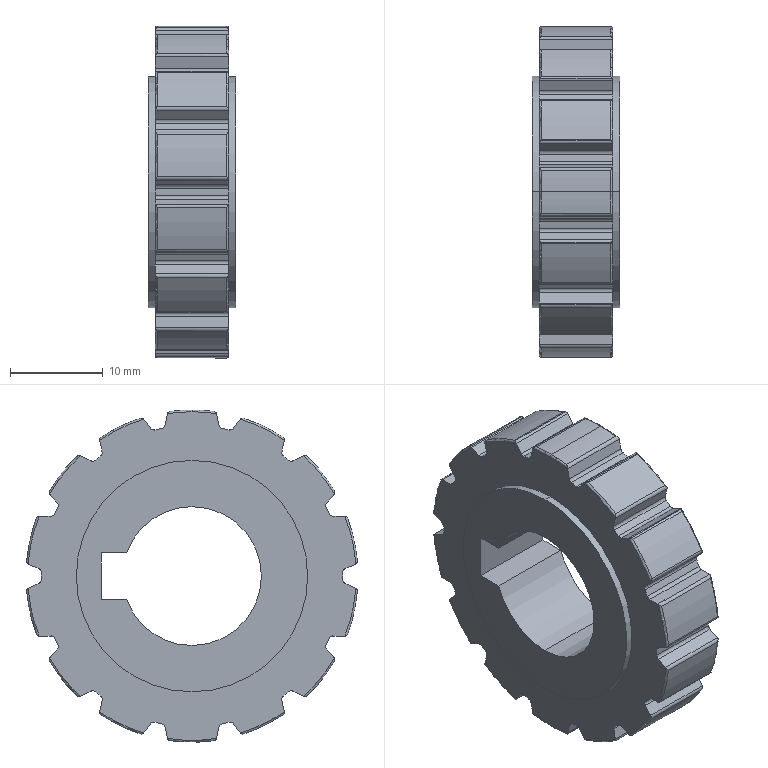Part | SolidWorks | features ICE 3, Cut 2, Chamfer 1, CirPattern 1, Fillet 1, RefAxis 1, Revolution 1 | 1 solid | 169 faces | box 9.48 x 35.738 x 35.892 mm | volume 6598 mm3 | cylinder 104 | plane 35 | torus 30 | commonest cylinder face diameters 0.76 x34 0.82 x34 35.892 x15 32.592 x14 25 x4 15 x3